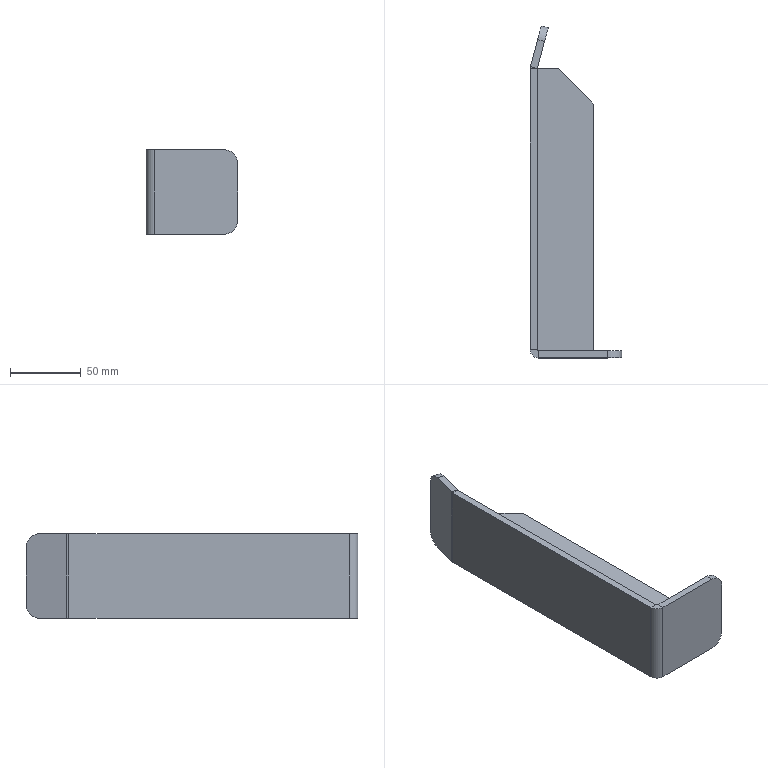Part | SolidWorks | features Fillet 1, FlatPattern 1, Gusset 1, SMBaseFlange 1, SheetMetal 1 | 2 solids | 33 faces | box 65 x 235.272 x 60 mm | volume 126254 mm3 | plane 25 | cylinder 8 | commonest cylinder face diameters 20 x4 2 x2 12 x2
STEP:
#1=CARTESIAN_POINT('',(0.,199.868,60.));
#2=VERTEX_POINT('',#1);
#3=CARTESIAN_POINT('',(-5.,199.868,60.));
#4=VERTEX_POINT('',#3);
#5=CARTESIAN_POINT('',(0.,199.868,60.));
#6=DIRECTION('',(-1.,0.,0.));
#7=VECTOR('',#6,1000.);
#8=LINE('',#5,#7);
#9=EDGE_CURVE('',#2,#4,#8,.T.);
#10=ORIENTED_EDGE('',*,*,#9,.F.);
#11=CARTESIAN_POINT('',(0.03407,200.127,60.));
#12=VERTEX_POINT('',#11);
#13=CARTESIAN_POINT('',(1.,199.868,60.));
#14=DIRECTION('',(0.,0.,1.));
#15=DIRECTION('',(-1.,0.,0.));
#16=AXIS2_PLACEMENT_3D('',#13,#14,#15);
#17=CIRCLE('',#16,1.);
#18=EDGE_CURVE('',#12,#2,#17,.T.);
#19=ORIENTED_EDGE('',*,*,#18,.F.);
#20=CARTESIAN_POINT('',(-4.796,201.421,60.));
#21=VERTEX_POINT('',#20);
#22=CARTESIAN_POINT('',(-4.796,201.421,60.));
#23=DIRECTION('',(0.9659,-0.2588,0.));
#24=VECTOR('',#23,1000.);
#25=LINE('',#22,#24);
#26=EDGE_CURVE('',#21,#12,#25,.T.);
#27=ORIENTED_EDGE('',*,*,#26,.F.);
#28=CARTESIAN_POINT('',(1.,199.868,60.));
#29=DIRECTION('',(0.,0.,1.));
#30=DIRECTION('',(1.,0.,0.));
#31=AXIS2_PLACEMENT_3D('',#28,#29,#30);
#32=CIRCLE('',#31,6.);
#33=EDGE_CURVE('',#21,#4,#32,.T.);
#34=ORIENTED_EDGE('',*,*,#33,.T.);
#35=EDGE_LOOP('',(#10,#19,#27,#34));
#36=FACE_OUTER_BOUND('',#35,.T.);
#37=CARTESIAN_POINT('',(0.,199.868,60.));
#38=DIRECTION('',(0.,0.,1.));
#39=DIRECTION('',(1.,0.,0.));
#40=AXIS2_PLACEMENT_3D('',#37,#38,#39);
#41=PLANE('',#40);
#42=ADVANCED_FACE('',(#36),#41,.T.);
#43=CARTESIAN_POINT('',(0.,1.,60.));
#44=VERTEX_POINT('',#43);
#45=CARTESIAN_POINT('',(0.,200.,60.));
#46=DIRECTION('',(0.,-1.,0.));
#47=VECTOR('',#46,1000.);
#48=LINE('',#45,#47);
#49=EDGE_CURVE('',#2,#44,#48,.T.);
#50=ORIENTED_EDGE('',*,*,#49,.F.);
#51=ORIENTED_EDGE('',*,*,#9,.T.);
#52=CARTESIAN_POINT('',(-5.,1.,60.));
#53=VERTEX_POINT('',#52);
#54=CARTESIAN_POINT('',(-5.,200.,60.));
#55=DIRECTION('',(0.,-1.,0.));
#56=VECTOR('',#55,1000.);
#57=LINE('',#54,#56);
#58=EDGE_CURVE('',#4,#53,#57,.T.);
#59=ORIENTED_EDGE('',*,*,#58,.T.);
#60=CARTESIAN_POINT('',(-5.,1.,60.));
#61=DIRECTION('',(1.,0.,0.));
#62=VECTOR('',#61,1000.);
#63=LINE('',#60,#62);
#64=EDGE_CURVE('',#53,#44,#63,.T.);
#65=ORIENTED_EDGE('',*,*,#64,.T.);
#66=EDGE_LOOP('',(#50,#51,#59,#65));
#67=FACE_OUTER_BOUND('',#66,.T.);
#68=CARTESIAN_POINT('',(-4.796,201.421,60.));
#69=DIRECTION('',(0.,0.,1.));
#70=DIRECTION('',(1.,0.,0.));
#71=AXIS2_PLACEMENT_3D('',#68,#69,#70);
#72=PLANE('',#71);
#73=ADVANCED_FACE('',(#67),#72,.T.);
#74=CARTESIAN_POINT('',(0.03407,200.127,0.));
#75=VERTEX_POINT('',#74);
#76=CARTESIAN_POINT('',(-4.796,201.421,0.));
#77=VERTEX_POINT('',#76);
#78=CARTESIAN_POINT('',(0.03407,200.127,0.));
#79=DIRECTION('',(-0.9659,0.2588,0.));
#80=VECTOR('',#79,1000.);
#81=LINE('',#78,#80);
#82=EDGE_CURVE('',#75,#77,#81,.T.);
#83=ORIENTED_EDGE('',*,*,#82,.F.);
#84=CARTESIAN_POINT('',(0.,199.868,0.));
#85=VERTEX_POINT('',#84);
#86=CARTESIAN_POINT('',(1.,199.868,0.));
#87=DIRECTION('',(0.,0.,1.));
#88=DIRECTION('',(-1.,0.,0.));
#89=AXIS2_PLACEMENT_3D('',#86,#87,#88);
#90=CIRCLE('',#89,1.);
#91=EDGE_CURVE('',#75,#85,#90,.T.);
#92=ORIENTED_EDGE('',*,*,#91,.T.);
#93=CARTESIAN_POINT('',(-5.,199.868,0.));
#94=VERTEX_POINT('',#93);
#95=CARTESIAN_POINT('',(-5.,199.868,0.));
#96=DIRECTION('',(1.,0.,0.));
#97=VECTOR('',#96,1000.);
#98=LINE('',#95,#97);
#99=EDGE_CURVE('',#94,#85,#98,.T.);
#100=ORIENTED_EDGE('',*,*,#99,.F.);
#101=CARTESIAN_POINT('',(1.,199.868,0.));
#102=DIRECTION('',(0.,0.,1.));
#103=DIRECTION('',(1.,0.,0.));
#104=AXIS2_PLACEMENT_3D('',#101,#102,#103);
#105=CIRCLE('',#104,6.);
#106=EDGE_CURVE('',#77,#94,#105,.T.);
#107=ORIENTED_EDGE('',*,*,#106,.F.);
#108=EDGE_LOOP('',(#83,#92,#100,#107));
#109=FACE_OUTER_BOUND('',#108,.T.);
#110=CARTESIAN_POINT('',(0.03407,200.127,0.));
#111=DIRECTION('',(0.,0.,-1.));
#112=DIRECTION('',(-1.,0.,0.));
#113=AXIS2_PLACEMENT_3D('',#110,#111,#112);
#114=PLANE('',#113);
#115=ADVANCED_FACE('',(#109),#114,.T.);
#116=CARTESIAN_POINT('',(0.3468,220.613,0.));
#117=VERTEX_POINT('',#116);
#118=CARTESIAN_POINT('',(-4.83,201.294,0.));
#119=DIRECTION('',(-0.2588,-0.9659,0.));
#120=VECTOR('',#119,1000.);
#121=LINE('',#118,#120);
#122=EDGE_CURVE('',#117,#77,#121,.T.);
#123=ORIENTED_EDGE('',*,*,#122,.F.);
#124=CARTESIAN_POINT('',(5.176,219.319,0.));
#125=VERTEX_POINT('',#124);
#126=CARTESIAN_POINT('',(0.5442,220.56,0.));
#127=DIRECTION('',(0.9659,-0.2588,0.));
#128=VECTOR('',#127,1000.);
#129=LINE('',#126,#128);
#130=EDGE_CURVE('',#117,#125,#129,.T.);
#131=ORIENTED_EDGE('',*,*,#130,.T.);
#132=CARTESIAN_POINT('',(0.,200.,0.));
#133=DIRECTION('',(-0.2588,-0.9659,0.));
#134=VECTOR('',#133,1000.);
#135=LINE('',#132,#134);
#136=EDGE_CURVE('',#125,#75,#135,.T.);
#137=ORIENTED_EDGE('',*,*,#136,.T.);
#138=ORIENTED_EDGE('',*,*,#82,.T.);
#139=EDGE_LOOP('',(#123,#131,#137,#138));
#140=FACE_OUTER_BOUND('',#139,.T.);
#141=CARTESIAN_POINT('',(-5.,199.868,0.));
#142=DIRECTION('',(0.,0.,-1.));
#143=DIRECTION('',(-1.,0.,0.));
#144=AXIS2_PLACEMENT_3D('',#141,#142,#143);
#145=PLANE('',#144);
#146=ADVANCED_FACE('',(#140),#145,.T.);
#147=CARTESIAN_POINT('',(1.,0.,60.));
#148=VERTEX_POINT('',#147);
#149=CARTESIAN_POINT('',(1.,-5.,60.));
#150=VERTEX_POINT('',#149);
#151=CARTESIAN_POINT('',(1.,0.,60.));
#152=DIRECTION('',(0.,-1.,0.));
#153=VECTOR('',#152,1000.);
#154=LINE('',#151,#153);
#155=EDGE_CURVE('',#148,#150,#154,.T.);
#156=ORIENTED_EDGE('',*,*,#155,.F.);
#157=CARTESIAN_POINT('',(1.,1.,60.));
#158=DIRECTION('',(0.,0.,1.));
#159=DIRECTION('',(-1.,0.,0.));
#160=AXIS2_PLACEMENT_3D('',#157,#158,#159);
#161=CIRCLE('',#160,1.);
#162=EDGE_CURVE('',#44,#148,#161,.T.);
#163=ORIENTED_EDGE('',*,*,#162,.F.);
#164=ORIENTED_EDGE('',*,*,#64,.F.);
#165=CARTESIAN_POINT('',(1.,1.,60.));
#166=DIRECTION('',(0.,0.,1.));
#167=DIRECTION('',(1.,0.,0.));
#168=AXIS2_PLACEMENT_3D('',#165,#166,#167);
#169=CIRCLE('',#168,6.);
#170=EDGE_CURVE('',#53,#150,#169,.T.);
#171=ORIENTED_EDGE('',*,*,#170,.T.);
#172=EDGE_LOOP('',(#156,#163,#164,#171));
#173=FACE_OUTER_BOUND('',#172,.T.);
#174=CARTESIAN_POINT('',(1.,0.,60.));
#175=DIRECTION('',(0.,0.,1.));
#176=DIRECTION('',(1.,0.,0.));
#177=AXIS2_PLACEMENT_3D('',#174,#175,#176);
#178=PLANE('',#177);
#179=ADVANCED_FACE('',(#173),#178,.T.);
#180=CARTESIAN_POINT('',(50.,-5.,60.));
#181=VERTEX_POINT('',#180);
#182=CARTESIAN_POINT('',(0.,-5.,60.));
#183=DIRECTION('',(1.,0.,0.));
#184=VECTOR('',#183,1000.);
#185=LINE('',#182,#184);
#186=EDGE_CURVE('',#150,#181,#185,.T.);
#187=ORIENTED_EDGE('',*,*,#186,.T.);
#188=CARTESIAN_POINT('',(50.,0.,60.));
#189=VERTEX_POINT('',#188);
#190=CARTESIAN_POINT('',(50.,1.,60.));
#191=DIRECTION('',(0.,1.,0.));
#192=VECTOR('',#191,1000.);
#193=LINE('',#190,#192);
#194=EDGE_CURVE('',#181,#189,#193,.T.);
#195=ORIENTED_EDGE('',*,*,#194,.T.);
#196=CARTESIAN_POINT('',(0.,0.,60.));
#197=DIRECTION('',(1.,0.,0.));
#198=VECTOR('',#197,1000.);
#199=LINE('',#196,#198);
#200=EDGE_CURVE('',#148,#189,#199,.T.);
#201=ORIENTED_EDGE('',*,*,#200,.F.);
#202=ORIENTED_EDGE('',*,*,#155,.T.);
#203=EDGE_LOOP('',(#187,#195,#201,#202));
#204=FACE_OUTER_BOUND('',#203,.T.);
#205=CARTESIAN_POINT('',(-5.,1.,60.));
#206=DIRECTION('',(0.,0.,1.));
#207=DIRECTION('',(1.,0.,0.));
#208=AXIS2_PLACEMENT_3D('',#205,#206,#207);
#209=PLANE('',#208);
#210=ADVANCED_FACE('',(#204),#209,.T.);
#211=CARTESIAN_POINT('',(0.,1.,0.));
#212=VERTEX_POINT('',#211);
#213=CARTESIAN_POINT('',(-5.,1.,0.));
#214=VERTEX_POINT('',#213);
#215=CARTESIAN_POINT('',(0.,1.,0.));
#216=DIRECTION('',(-1.,0.,0.));
#217=VECTOR('',#216,1000.);
#218=LINE('',#215,#217);
#219=EDGE_CURVE('',#212,#214,#218,.T.);
#220=ORIENTED_EDGE('',*,*,#219,.F.);
#221=CARTESIAN_POINT('',(1.,0.,0.));
#222=VERTEX_POINT('',#221);
#223=CARTESIAN_POINT('',(1.,1.,0.));
#224=DIRECTION('',(0.,0.,1.));
#225=DIRECTION('',(-1.,0.,0.));
#226=AXIS2_PLACEMENT_3D('',#223,#224,#225);
#227=CIRCLE('',#226,1.);
#228=EDGE_CURVE('',#212,#222,#227,.T.);
#229=ORIENTED_EDGE('',*,*,#228,.T.);
#230=CARTESIAN_POINT('',(1.,-5.,0.));
#231=VERTEX_POINT('',#230);
#232=CARTESIAN_POINT('',(1.,-5.,0.));
#233=DIRECTION('',(0.,1.,0.));
#234=VECTOR('',#233,1000.);
#235=LINE('',#232,#234);
#236=EDGE_CURVE('',#231,#222,#235,.T.);
#237=ORIENTED_EDGE('',*,*,#236,.F.);
#238=CARTESIAN_POINT('',(1.,1.,0.));
#239=DIRECTION('',(0.,0.,1.));
#240=DIRECTION('',(1.,0.,0.));
#241=AXIS2_PLACEMENT_3D('',#238,#239,#240);
#242=CIRCLE('',#241,6.);
#243=EDGE_CURVE('',#214,#231,#242,.T.);
#244=ORIENTED_EDGE('',*,*,#243,.F.);
#245=EDGE_LOOP('',(#220,#229,#237,#244));
#246=FACE_OUTER_BOUND('',#245,.T.);
#247=CARTESIAN_POINT('',(0.,1.,0.));
#248=DIRECTION('',(0.,0.,-1.));
#249=DIRECTION('',(-1.,0.,0.));
#250=AXIS2_PLACEMENT_3D('',#247,#248,#249);
#251=PLANE('',#250);
#252=ADVANCED_FACE('',(#246),#251,.T.);
#253=CARTESIAN_POINT('',(0.,200.,0.));
#254=DIRECTION('',(0.,-1.,0.));
#255=VECTOR('',#254,1000.);
#256=LINE('',#253,#255);
#257=EDGE_CURVE('',#85,#212,#256,.T.);
#258=ORIENTED_EDGE('',*,*,#257,.T.);
#259=ORIENTED_EDGE('',*,*,#219,.T.);
#260=CARTESIAN_POINT('',(-5.,200.,0.));
#261=DIRECTION('',(0.,-1.,0.));
#262=VECTOR('',#261,1000.);
#263=LINE('',#260,#262);
#264=EDGE_CURVE('',#94,#214,#263,.T.);
#265=ORIENTED_EDGE('',*,*,#264,.F.);
#266=ORIENTED_EDGE('',*,*,#99,.T.);
#267=EDGE_LOOP('',(#258,#259,#265,#266));
#268=FACE_OUTER_BOUND('',#267,.T.);
#269=CARTESIAN_POINT('',(1.,-5.,0.));
#270=DIRECTION('',(0.,0.,-1.));
#271=DIRECTION('',(-1.,0.,0.));
#272=AXIS2_PLACEMENT_3D('',#269,#270,#271);
#273=PLANE('',#272);
#274=ADVANCED_FACE('',(#268),#273,.T.);
#275=CARTESIAN_POINT('',(50.,-5.,0.));
#276=VERTEX_POINT('',#275);
#277=CARTESIAN_POINT('',(0.,-5.,0.));
#278=DIRECTION('',(1.,0.,0.));
#279=VECTOR('',#278,1000.);
#280=LINE('',#277,#279);
#281=EDGE_CURVE('',#231,#276,#280,.T.);
#282=ORIENTED_EDGE('',*,*,#281,.T.);
#283=CARTESIAN_POINT('',(60.,-5.,10.));
#284=VERTEX_POINT('',#283);
#285=CARTESIAN_POINT('',(50.,-5.,10.));
#286=DIRECTION('',(0.,-1.,0.));
#287=DIRECTION('',(0.,0.,1.));
#288=AXIS2_PLACEMENT_3D('',#285,#286,#287);
#289=CIRCLE('',#288,10.);
#290=EDGE_CURVE('',#276,#284,#289,.T.);
#291=ORIENTED_EDGE('',*,*,#290,.T.);
#292=CARTESIAN_POINT('',(60.,-5.,50.));
#293=VERTEX_POINT('',#292);
#294=CARTESIAN_POINT('',(60.,-5.,60.));
#295=DIRECTION('',(0.,0.,-1.));
#296=VECTOR('',#295,1000.);
#297=LINE('',#294,#296);
#298=EDGE_CURVE('',#293,#284,#297,.T.);
#299=ORIENTED_EDGE('',*,*,#298,.F.);
#300=CARTESIAN_POINT('',(50.,-5.,50.));
#301=DIRECTION('',(0.,-1.,0.));
#302=DIRECTION('',(0.,0.,1.));
#303=AXIS2_PLACEMENT_3D('',#300,#301,#302);
#304=CIRCLE('',#303,10.);
#305=EDGE_CURVE('',#293,#181,#304,.T.);
#306=ORIENTED_EDGE('',*,*,#305,.T.);
#307=ORIENTED_EDGE('',*,*,#186,.F.);
#308=CARTESIAN_POINT('',(1.,-5.,60.));
#309=DIRECTION('',(0.,0.,-1.));
#310=VECTOR('',#309,1000.);
#311=LINE('',#308,#310);
#312=EDGE_CURVE('',#150,#231,#311,.T.);
#313=ORIENTED_EDGE('',*,*,#312,.T.);
#314=EDGE_LOOP('',(#282,#291,#299,#306,#307,#313));
#315=FACE_OUTER_BOUND('',#314,.T.);
#316=CARTESIAN_POINT('',(0.,-5.,60.));
#317=DIRECTION('',(0.,1.,0.));
#318=DIRECTION('',(0.,0.,1.));
#319=AXIS2_PLACEMENT_3D('',#316,#317,#318);
#320=PLANE('',#319);
#321=ADVANCED_FACE('',(#315),#320,.F.);
#322=ORIENTED_EDGE('',*,*,#298,.T.);
#323=CARTESIAN_POINT('',(60.,0.,10.));
#324=VERTEX_POINT('',#323);
#325=CARTESIAN_POINT('',(60.,0.,10.));
#326=DIRECTION('',(0.,1.,0.));
#327=VECTOR('',#326,1000.);
#328=LINE('',#325,#327);
#329=EDGE_CURVE('',#284,#324,#328,.T.);
#330=ORIENTED_EDGE('',*,*,#329,.T.);
#331=CARTESIAN_POINT('',(60.,0.,50.));
#332=VERTEX_POINT('',#331);
#333=CARTESIAN_POINT('',(60.,0.,60.));
#334=DIRECTION('',(0.,0.,-1.));
#335=VECTOR('',#334,1000.);
#336=LINE('',#333,#335);
#337=EDGE_CURVE('',#332,#324,#336,.T.);
#338=ORIENTED_EDGE('',*,*,#337,.F.);
#339=CARTESIAN_POINT('',(60.,0.,50.));
#340=DIRECTION('',(0.,-1.,0.));
#341=VECTOR('',#340,1000.);
#342=LINE('',#339,#341);
#343=EDGE_CURVE('',#332,#293,#342,.T.);
#344=ORIENTED_EDGE('',*,*,#343,.T.);
#345=EDGE_LOOP('',(#322,#330,#338,#344));
#346=FACE_OUTER_BOUND('',#345,.T.);
#347=CARTESIAN_POINT('',(60.,0.,60.));
#348=DIRECTION('',(1.,0.,0.));
#349=DIRECTION('',(0.,0.,-1.));
#350=AXIS2_PLACEMENT_3D('',#347,#348,#349);
#351=PLANE('',#350);
#352=ADVANCED_FACE('',(#346),#351,.T.);
#353=ORIENTED_EDGE('',*,*,#337,.T.);
#354=CARTESIAN_POINT('',(50.,0.,0.));
#355=VERTEX_POINT('',#354);
#356=CARTESIAN_POINT('',(50.,0.,10.));
#357=DIRECTION('',(0.,1.,0.));
#358=DIRECTION('',(0.,0.,1.));
#359=AXIS2_PLACEMENT_3D('',#356,#357,#358);
#360=CIRCLE('',#359,10.);
#361=EDGE_CURVE('',#324,#355,#360,.T.);
#362=ORIENTED_EDGE('',*,*,#361,.T.);
#363=CARTESIAN_POINT('',(0.,0.,0.));
#364=DIRECTION('',(1.,0.,0.));
#365=VECTOR('',#364,1000.);
#366=LINE('',#363,#365);
#367=EDGE_CURVE('',#222,#355,#366,.T.);
#368=ORIENTED_EDGE('',*,*,#367,.F.);
#369=CARTESIAN_POINT('',(1.,0.,60.));
#370=DIRECTION('',(0.,0.,-1.));
#371=VECTOR('',#370,1000.);
#372=LINE('',#369,#371);
#373=EDGE_CURVE('',#148,#222,#372,.T.);
#374=ORIENTED_EDGE('',*,*,#373,.F.);
#375=ORIENTED_EDGE('',*,*,#200,.T.);
#376=CARTESIAN_POINT('',(50.,0.,50.));
#377=DIRECTION('',(0.,1.,0.));
#378=DIRECTION('',(0.,0.,1.));
#379=AXIS2_PLACEMENT_3D('',#376,#377,#378);
#380=CIRCLE('',#379,10.);
#381=EDGE_CURVE('',#189,#332,#380,.T.);
#382=ORIENTED_EDGE('',*,*,#381,.T.);
#383=EDGE_LOOP('',(#353,#362,#368,#374,#375,#382));
#384=FACE_OUTER_BOUND('',#383,.T.);
#385=CARTESIAN_POINT('',(0.,0.,60.));
#386=DIRECTION('',(0.,1.,0.));
#387=DIRECTION('',(0.,0.,1.));
#388=AXIS2_PLACEMENT_3D('',#385,#386,#387);
#389=PLANE('',#388);
#390=ADVANCED_FACE('',(#384),#389,.T.);
#391=ORIENTED_EDGE('',*,*,#228,.F.);
#392=CARTESIAN_POINT('',(0.,1.,60.));
#393=DIRECTION('',(0.,0.,-1.));
#394=VECTOR('',#393,1000.);
#395=LINE('',#392,#394);
#396=EDGE_CURVE('',#44,#212,#395,.T.);
#397=ORIENTED_EDGE('',*,*,#396,.F.);
#398=ORIENTED_EDGE('',*,*,#162,.T.);
#399=ORIENTED_EDGE('',*,*,#373,.T.);
#400=EDGE_LOOP('',(#391,#397,#398,#399));
#401=FACE_OUTER_BOUND('',#400,.T.);
#402=CARTESIAN_POINT('',(1.,1.,60.));
#403=DIRECTION('',(0.,0.,-1.));
#404=DIRECTION('',(-1.,0.,0.));
#405=AXIS2_PLACEMENT_3D('',#402,#403,#404);
#406=CYLINDRICAL_SURFACE('',#405,1.);
#407=ADVANCED_FACE('',(#401),#406,.F.);
#408=ORIENTED_EDGE('',*,*,#257,.F.);
#409=CARTESIAN_POINT('',(0.,199.868,60.));
#410=DIRECTION('',(0.,0.,-1.));
#411=VECTOR('',#410,1000.);
#412=LINE('',#409,#411);
#413=EDGE_CURVE('',#2,#85,#412,.T.);
#414=ORIENTED_EDGE('',*,*,#413,.F.);
#415=ORIENTED_EDGE('',*,*,#49,.T.);
#416=ORIENTED_EDGE('',*,*,#396,.T.);
#417=EDGE_LOOP('',(#408,#414,#415,#416));
#418=FACE_OUTER_BOUND('',#417,.T.);
#419=CARTESIAN_POINT('',(0.,200.,60.));
#420=DIRECTION('',(1.,0.,0.));
#421=DIRECTION('',(0.,1.,0.));
#422=AXIS2_PLACEMENT_3D('',#419,#420,#421);
#423=PLANE('',#422);
#424=ADVANCED_FACE('',(#418),#423,.T.);
#425=ORIENTED_EDGE('',*,*,#91,.F.);
#426=CARTESIAN_POINT('',(0.03407,200.127,60.));
#427=DIRECTION('',(0.,0.,-1.));
#428=VECTOR('',#427,1000.);
#429=LINE('',#426,#428);
#430=EDGE_CURVE('',#12,#75,#429,.T.);
#431=ORIENTED_EDGE('',*,*,#430,.F.);
#432=ORIENTED_EDGE('',*,*,#18,.T.);
#433=ORIENTED_EDGE('',*,*,#413,.T.);
#434=EDGE_LOOP('',(#425,#431,#432,#433));
#435=FACE_OUTER_BOUND('',#434,.T.);
#436=CARTESIAN_POINT('',(1.,199.868,60.));
#437=DIRECTION('',(0.,0.,-1.));
#438=DIRECTION('',(-1.,0.,0.));
#439=AXIS2_PLACEMENT_3D('',#436,#437,#438);
#440=CYLINDRICAL_SURFACE('',#439,1.);
#441=ADVANCED_FACE('',(#435),#440,.F.);
#442=ORIENTED_EDGE('',*,*,#136,.F.);
#443=CARTESIAN_POINT('',(7.765,228.978,10.));
#444=VERTEX_POINT('',#443);
#445=CARTESIAN_POINT('',(5.176,219.319,10.));
#446=DIRECTION('',(0.9659,-0.2588,0.));
#447=DIRECTION('',(0.2588,0.9659,0.));
#448=AXIS2_PLACEMENT_3D('',#445,#446,#447);
#449=CIRCLE('',#448,10.);
#450=EDGE_CURVE('',#125,#444,#449,.T.);
#451=ORIENTED_EDGE('',*,*,#450,.T.);
#452=CARTESIAN_POINT('',(7.765,228.978,50.));
#453=VERTEX_POINT('',#452);
#454=CARTESIAN_POINT('',(7.765,228.978,60.));
#455=DIRECTION('',(0.,0.,-1.));
#456=VECTOR('',#455,1000.);
#457=LINE('',#454,#456);
#458=EDGE_CURVE('',#453,#444,#457,.T.);
#459=ORIENTED_EDGE('',*,*,#458,.F.);
#460=CARTESIAN_POINT('',(5.176,219.319,60.));
#461=VERTEX_POINT('',#460);
#462=CARTESIAN_POINT('',(5.176,219.319,50.));
#463=DIRECTION('',(0.9659,-0.2588,0.));
#464=DIRECTION('',(0.2588,0.9659,0.));
#465=AXIS2_PLACEMENT_3D('',#462,#463,#464);
#466=CIRCLE('',#465,10.);
#467=EDGE_CURVE('',#453,#461,#466,.T.);
#468=ORIENTED_EDGE('',*,*,#467,.T.);
#469=CARTESIAN_POINT('',(0.,200.,60.));
#470=DIRECTION('',(-0.2588,-0.9659,0.));
#471=VECTOR('',#470,1000.);
#472=LINE('',#469,#471);
#473=EDGE_CURVE('',#461,#12,#472,.T.);
#474=ORIENTED_EDGE('',*,*,#473,.T.);
#475=ORIENTED_EDGE('',*,*,#430,.T.);
#476=EDGE_LOOP('',(#442,#451,#459,#468,#474,#475));
#477=FACE_OUTER_BOUND('',#476,.T.);
#478=CARTESIAN_POINT('',(0.,200.,60.));
#479=DIRECTION('',(0.9659,-0.2588,0.));
#480=DIRECTION('',(0.2588,0.9659,0.));
#481=AXIS2_PLACEMENT_3D('',#478,#479,#480);
#482=PLANE('',#481);
#483=ADVANCED_FACE('',(#477),#482,.T.);
#484=ORIENTED_EDGE('',*,*,#458,.T.);
#485=CARTESIAN_POINT('',(2.935,230.272,10.));
#486=VERTEX_POINT('',#485);
#487=CARTESIAN_POINT('',(2.935,230.272,10.));
#488=DIRECTION('',(-0.9659,0.2588,0.));
#489=VECTOR('',#488,1000.);
#490=LINE('',#487,#489);
#491=EDGE_CURVE('',#444,#486,#490,.T.);
#492=ORIENTED_EDGE('',*,*,#491,.T.);
#493=CARTESIAN_POINT('',(2.935,230.272,50.));
#494=VERTEX_POINT('',#493);
#495=CARTESIAN_POINT('',(2.935,230.272,60.));
#496=DIRECTION('',(0.,0.,-1.));
#497=VECTOR('',#496,1000.);
#498=LINE('',#495,#497);
#499=EDGE_CURVE('',#494,#486,#498,.T.);
#500=ORIENTED_EDGE('',*,*,#499,.F.);
#501=CARTESIAN_POINT('',(7.765,228.978,50.));
#502=DIRECTION('',(0.9659,-0.2588,0.));
#503=VECTOR('',#502,1000.);
#504=LINE('',#501,#503);
#505=EDGE_CURVE('',#494,#453,#504,.T.);
#506=ORIENTED_EDGE('',*,*,#505,.T.);
#507=EDGE_LOOP('',(#484,#492,#500,#506));
#508=FACE_OUTER_BOUND('',#507,.T.);
#509=CARTESIAN_POINT('',(2.935,230.272,60.));
#510=DIRECTION('',(0.2588,0.9659,0.));
#511=DIRECTION('',(-0.9659,0.2588,0.));
#512=AXIS2_PLACEMENT_3D('',#509,#510,#511);
#513=PLANE('',#512);
#514=ADVANCED_FACE('',(#508),#513,.T.);
#515=ORIENTED_EDGE('',*,*,#499,.T.);
#516=CARTESIAN_POINT('',(0.3468,220.613,10.));
#517=DIRECTION('',(-0.9659,0.2588,0.));
#518=DIRECTION('',(0.2588,0.9659,0.));
#519=AXIS2_PLACEMENT_3D('',#516,#517,#518);
#520=CIRCLE('',#519,10.);
#521=EDGE_CURVE('',#486,#117,#520,.T.);
#522=ORIENTED_EDGE('',*,*,#521,.T.);
#523=ORIENTED_EDGE('',*,*,#122,.T.);
#524=CARTESIAN_POINT('',(-4.796,201.421,60.));
#525=DIRECTION('',(0.,0.,-1.));
#526=VECTOR('',#525,1000.);
#527=LINE('',#524,#526);
#528=EDGE_CURVE('',#21,#77,#527,.T.);
#529=ORIENTED_EDGE('',*,*,#528,.F.);
#530=CARTESIAN_POINT('',(0.3468,220.613,60.));
#531=VERTEX_POINT('',#530);
#532=CARTESIAN_POINT('',(-4.83,201.294,60.));
#533=DIRECTION('',(-0.2588,-0.9659,0.));
#534=VECTOR('',#533,1000.);
#535=LINE('',#532,#534);
#536=EDGE_CURVE('',#531,#21,#535,.T.);
#537=ORIENTED_EDGE('',*,*,#536,.F.);
#538=CARTESIAN_POINT('',(0.3468,220.613,50.));
#539=DIRECTION('',(-0.9659,0.2588,0.));
#540=DIRECTION('',(0.2588,0.9659,0.));
#541=AXIS2_PLACEMENT_3D('',#538,#539,#540);
#542=CIRCLE('',#541,10.);
#543=EDGE_CURVE('',#531,#494,#542,.T.);
#544=ORIENTED_EDGE('',*,*,#543,.T.);
#545=EDGE_LOOP('',(#515,#522,#523,#529,#537,#544));
#546=FACE_OUTER_BOUND('',#545,.T.);
#547=CARTESIAN_POINT('',(-4.83,201.294,60.));
#548=DIRECTION('',(0.9659,-0.2588,0.));
#549=DIRECTION('',(0.2588,0.9659,0.));
#550=AXIS2_PLACEMENT_3D('',#547,#548,#549);
#551=PLANE('',#550);
#552=ADVANCED_FACE('',(#546),#551,.F.);
#553=ORIENTED_EDGE('',*,*,#106,.T.);
#554=CARTESIAN_POINT('',(-5.,199.868,60.));
#555=DIRECTION('',(0.,0.,-1.));
#556=VECTOR('',#555,1000.);
#557=LINE('',#554,#556);
#558=EDGE_CURVE('',#4,#94,#557,.T.);
#559=ORIENTED_EDGE('',*,*,#558,.F.);
#560=ORIENTED_EDGE('',*,*,#33,.F.);
#561=ORIENTED_EDGE('',*,*,#528,.T.);
#562=EDGE_LOOP('',(#553,#559,#560,#561));
#563=FACE_OUTER_BOUND('',#562,.T.);
#564=CARTESIAN_POINT('',(1.,199.868,60.));
#565=DIRECTION('',(0.,0.,-1.));
#566=DIRECTION('',(-1.,0.,0.));
#567=AXIS2_PLACEMENT_3D('',#564,#565,#566);
#568=CYLINDRICAL_SURFACE('',#567,6.);
#569=ADVANCED_FACE('',(#563),#568,.T.);
#570=ORIENTED_EDGE('',*,*,#264,.T.);
#571=CARTESIAN_POINT('',(-5.,1.,60.));
#572=DIRECTION('',(0.,0.,-1.));
#573=VECTOR('',#572,1000.);
#574=LINE('',#571,#573);
#575=EDGE_CURVE('',#53,#214,#574,.T.);
#576=ORIENTED_EDGE('',*,*,#575,.F.);
#577=ORIENTED_EDGE('',*,*,#58,.F.);
#578=ORIENTED_EDGE('',*,*,#558,.T.);
#579=EDGE_LOOP('',(#570,#576,#577,#578));
#580=FACE_OUTER_BOUND('',#579,.T.);
#581=CARTESIAN_POINT('',(-5.,200.,60.));
#582=DIRECTION('',(1.,0.,0.));
#583=DIRECTION('',(0.,1.,0.));
#584=AXIS2_PLACEMENT_3D('',#581,#582,#583);
#585=PLANE('',#584);
#586=ADVANCED_FACE('',(#580),#585,.F.);
#587=ORIENTED_EDGE('',*,*,#243,.T.);
#588=ORIENTED_EDGE('',*,*,#312,.F.);
#589=ORIENTED_EDGE('',*,*,#170,.F.);
#590=ORIENTED_EDGE('',*,*,#575,.T.);
#591=EDGE_LOOP('',(#587,#588,#589,#590));
#592=FACE_OUTER_BOUND('',#591,.T.);
#593=CARTESIAN_POINT('',(1.,1.,60.));
#594=DIRECTION('',(0.,0.,-1.));
#595=DIRECTION('',(-1.,0.,0.));
#596=AXIS2_PLACEMENT_3D('',#593,#594,#595);
#597=CYLINDRICAL_SURFACE('',#596,6.);
#598=ADVANCED_FACE('',(#592),#597,.T.);
#599=ORIENTED_EDGE('',*,*,#473,.F.);
#600=CARTESIAN_POINT('',(0.3468,220.613,60.));
#601=DIRECTION('',(-0.9659,0.2588,0.));
#602=VECTOR('',#601,1000.);
#603=LINE('',#600,#602);
#604=EDGE_CURVE('',#461,#531,#603,.T.);
#605=ORIENTED_EDGE('',*,*,#604,.T.);
#606=ORIENTED_EDGE('',*,*,#536,.T.);
#607=ORIENTED_EDGE('',*,*,#26,.T.);
#608=EDGE_LOOP('',(#599,#605,#606,#607));
#609=FACE_OUTER_BOUND('',#608,.T.);
#610=CARTESIAN_POINT('',(1.,1.,60.));
#611=DIRECTION('',(0.,0.,-1.));
#612=DIRECTION('',(-1.,0.,0.));
#613=AXIS2_PLACEMENT_3D('',#610,#611,#612);
#614=PLANE('',#613);
#615=ADVANCED_FACE('',(#609),#614,.F.);
#616=ORIENTED_EDGE('',*,*,#367,.T.);
#617=CARTESIAN_POINT('',(50.,1.,0.));
#618=DIRECTION('',(0.,-1.,0.));
#619=VECTOR('',#618,1000.);
#620=LINE('',#617,#619);
#621=EDGE_CURVE('',#355,#276,#620,.T.);
#622=ORIENTED_EDGE('',*,*,#621,.T.);
#623=ORIENTED_EDGE('',*,*,#281,.F.);
#624=ORIENTED_EDGE('',*,*,#236,.T.);
#625=EDGE_LOOP('',(#616,#622,#623,#624));
#626=FACE_OUTER_BOUND('',#625,.T.);
#627=CARTESIAN_POINT('',(1.,1.,0.));
#628=DIRECTION('',(0.,0.,-1.));
#629=DIRECTION('',(-1.,0.,0.));
#630=AXIS2_PLACEMENT_3D('',#627,#628,#629);
#631=PLANE('',#630);
#632=ADVANCED_FACE('',(#626),#631,.T.);
#633=ORIENTED_EDGE('',*,*,#361,.F.);
#634=ORIENTED_EDGE('',*,*,#329,.F.);
#635=ORIENTED_EDGE('',*,*,#290,.F.);
#636=ORIENTED_EDGE('',*,*,#621,.F.);
#637=EDGE_LOOP('',(#633,#634,#635,#636));
#638=FACE_OUTER_BOUND('',#637,.T.);
#639=CARTESIAN_POINT('',(50.,1.,10.));
#640=DIRECTION('',(0.,-1.,0.));
#641=DIRECTION('',(0.,0.,-1.));
#642=AXIS2_PLACEMENT_3D('',#639,#640,#641);
#643=CYLINDRICAL_SURFACE('',#642,10.);
#644=ADVANCED_FACE('',(#638),#643,.T.);
#645=ORIENTED_EDGE('',*,*,#381,.F.);
#646=ORIENTED_EDGE('',*,*,#194,.F.);
#647=ORIENTED_EDGE('',*,*,#305,.F.);
#648=ORIENTED_EDGE('',*,*,#343,.F.);
#649=EDGE_LOOP('',(#645,#646,#647,#648));
#650=FACE_OUTER_BOUND('',#649,.T.);
#651=CARTESIAN_POINT('',(50.,0.,50.));
#652=DIRECTION('',(0.,-1.,0.));
#653=DIRECTION('',(0.,0.,-1.));
#654=AXIS2_PLACEMENT_3D('',#651,#652,#653);
#655=CYLINDRICAL_SURFACE('',#654,10.);
#656=ADVANCED_FACE('',(#650),#655,.T.);
#657=ORIENTED_EDGE('',*,*,#521,.F.);
#658=ORIENTED_EDGE('',*,*,#491,.F.);
#659=ORIENTED_EDGE('',*,*,#450,.F.);
#660=ORIENTED_EDGE('',*,*,#130,.F.);
#661=EDGE_LOOP('',(#657,#658,#659,#660));
#662=FACE_OUTER_BOUND('',#661,.T.);
#663=CARTESIAN_POINT('',(0.5442,220.56,10.));
#664=DIRECTION('',(0.9659,-0.2588,0.));
#665=DIRECTION('',(0.2588,0.9659,0.));
#666=AXIS2_PLACEMENT_3D('',#663,#664,#665);
#667=CYLINDRICAL_SURFACE('',#666,10.);
#668=ADVANCED_FACE('',(#662),#667,.T.);
#669=ORIENTED_EDGE('',*,*,#543,.F.);
#670=ORIENTED_EDGE('',*,*,#604,.F.);
#671=ORIENTED_EDGE('',*,*,#467,.F.);
#672=ORIENTED_EDGE('',*,*,#505,.F.);
#673=EDGE_LOOP('',(#669,#670,#671,#672));
#674=FACE_OUTER_BOUND('',#673,.T.);
#675=CARTESIAN_POINT('',(0.3468,220.613,50.));
#676=DIRECTION('',(-0.9659,0.2588,0.));
#677=DIRECTION('',(-0.2588,-0.9659,0.));
#678=AXIS2_PLACEMENT_3D('',#675,#676,#677);
#679=CYLINDRICAL_SURFACE('',#678,10.);
#680=ADVANCED_FACE('',(#674),#679,.T.);
#681=CLOSED_SHELL('',(#42,#73,#115,#146,#179,#210,#252,#274,#321,#352,#390,#407,#424,#441,#483,#514,#552,#569,#586,#598,#615,#632,#644,#656,#668,#680));
#682=MANIFOLD_SOLID_BREP('',#681);
#683=CARTESIAN_POINT('',(0.,200.,32.5));
#684=VERTEX_POINT('',#683);
#685=CARTESIAN_POINT('',(15.,200.,32.5));
#686=VERTEX_POINT('',#685);
#687=CARTESIAN_POINT('',(0.,200.,32.5));
#688=DIRECTION('',(1.,0.,0.));
#689=VECTOR('',#688,1000.);
#690=LINE('',#687,#689);
#691=EDGE_CURVE('',#684,#686,#690,.T.);
#692=ORIENTED_EDGE('',*,*,#691,.T.);
#693=CARTESIAN_POINT('',(15.,200.,27.5));
#694=VERTEX_POINT('',#693);
#695=CARTESIAN_POINT('',(15.,200.,27.5));
#696=DIRECTION('',(0.,0.,1.));
#697=VECTOR('',#696,1000.);
#698=LINE('',#695,#697);
#699=EDGE_CURVE('',#694,#686,#698,.T.);
#700=ORIENTED_EDGE('',*,*,#699,.F.);
#701=CARTESIAN_POINT('',(0.,200.,27.5));
#702=VERTEX_POINT('',#701);
#703=CARTESIAN_POINT('',(0.,200.,27.5));
#704=DIRECTION('',(1.,0.,0.));
#705=VECTOR('',#704,1000.);
#706=LINE('',#703,#705);
#707=EDGE_CURVE('',#702,#694,#706,.T.);
#708=ORIENTED_EDGE('',*,*,#707,.F.);
#709=CARTESIAN_POINT('',(0.,200.,27.5));
#710=DIRECTION('',(0.,0.,1.));
#711=VECTOR('',#710,1000.);
#712=LINE('',#709,#711);
#713=EDGE_CURVE('',#702,#684,#712,.T.);
#714=ORIENTED_EDGE('',*,*,#713,.T.);
#715=EDGE_LOOP('',(#692,#700,#708,#714));
#716=FACE_OUTER_BOUND('',#715,.T.);
#717=CARTESIAN_POINT('',(0.,200.,27.5));
#718=DIRECTION('',(0.,-1.,0.));
#719=DIRECTION('',(0.,0.,-1.));
#720=AXIS2_PLACEMENT_3D('',#717,#718,#719);
#721=PLANE('',#720);
#722=ADVANCED_FACE('',(#716),#721,.F.);
#723=CARTESIAN_POINT('',(40.,175.,32.5));
#724=VERTEX_POINT('',#723);
#725=CARTESIAN_POINT('',(15.,200.,32.5));
#726=DIRECTION('',(0.7071,-0.7071,0.));
#727=VECTOR('',#726,1000.);
#728=LINE('',#725,#727);
#729=EDGE_CURVE('',#686,#724,#728,.T.);
#730=ORIENTED_EDGE('',*,*,#729,.T.);
#731=CARTESIAN_POINT('',(40.,175.,27.5));
#732=VERTEX_POINT('',#731);
#733=CARTESIAN_POINT('',(40.,175.,27.5));
#734=DIRECTION('',(0.,0.,1.));
#735=VECTOR('',#734,1000.);
#736=LINE('',#733,#735);
#737=EDGE_CURVE('',#732,#724,#736,.T.);
#738=ORIENTED_EDGE('',*,*,#737,.F.);
#739=CARTESIAN_POINT('',(15.,200.,27.5));
#740=DIRECTION('',(0.7071,-0.7071,0.));
#741=VECTOR('',#740,1000.);
#742=LINE('',#739,#741);
#743=EDGE_CURVE('',#694,#732,#742,.T.);
#744=ORIENTED_EDGE('',*,*,#743,.F.);
#745=ORIENTED_EDGE('',*,*,#699,.T.);
#746=EDGE_LOOP('',(#730,#738,#744,#745));
#747=FACE_OUTER_BOUND('',#746,.T.);
#748=CARTESIAN_POINT('',(15.,200.,27.5));
#749=DIRECTION('',(-0.7071,-0.7071,0.));
#750=DIRECTION('',(0.7071,-0.7071,0.));
#751=AXIS2_PLACEMENT_3D('',#748,#749,#750);
#752=PLANE('',#751);
#753=ADVANCED_FACE('',(#747),#752,.F.);
#754=CARTESIAN_POINT('',(40.,0.,32.5));
#755=VERTEX_POINT('',#754);
#756=CARTESIAN_POINT('',(40.,0.,32.5));
#757=DIRECTION('',(0.,-1.,0.));
#758=VECTOR('',#757,1000.);
#759=LINE('',#756,#758);
#760=EDGE_CURVE('',#724,#755,#759,.T.);
#761=ORIENTED_EDGE('',*,*,#760,.T.);
#762=CARTESIAN_POINT('',(40.,0.,27.5));
#763=VERTEX_POINT('',#762);
#764=CARTESIAN_POINT('',(40.,0.,27.5));
#765=DIRECTION('',(0.,0.,1.));
#766=VECTOR('',#765,1000.);
#767=LINE('',#764,#766);
#768=EDGE_CURVE('',#763,#755,#767,.T.);
#769=ORIENTED_EDGE('',*,*,#768,.F.);
#770=CARTESIAN_POINT('',(40.,0.,27.5));
#771=DIRECTION('',(0.,-1.,0.));
#772=VECTOR('',#771,1000.);
#773=LINE('',#770,#772);
#774=EDGE_CURVE('',#732,#763,#773,.T.);
#775=ORIENTED_EDGE('',*,*,#774,.F.);
#776=ORIENTED_EDGE('',*,*,#737,.T.);
#777=EDGE_LOOP('',(#761,#769,#775,#776));
#778=FACE_OUTER_BOUND('',#777,.T.);
#779=CARTESIAN_POINT('',(40.,0.,27.5));
#780=DIRECTION('',(-1.,0.,0.));
#781=DIRECTION('',(0.,0.,1.));
#782=AXIS2_PLACEMENT_3D('',#779,#780,#781);
#783=PLANE('',#782);
#784=ADVANCED_FACE('',(#778),#783,.F.);
#785=CARTESIAN_POINT('',(0.,0.,32.5));
#786=VERTEX_POINT('',#785);
#787=CARTESIAN_POINT('',(0.,0.,32.5));
#788=DIRECTION('',(-1.,0.,0.));
#789=VECTOR('',#788,1000.);
#790=LINE('',#787,#789);
#791=EDGE_CURVE('',#755,#786,#790,.T.);
#792=ORIENTED_EDGE('',*,*,#791,.T.);
#793=CARTESIAN_POINT('',(0.,0.,27.5));
#794=VERTEX_POINT('',#793);
#795=CARTESIAN_POINT('',(0.,0.,27.5));
#796=DIRECTION('',(0.,0.,1.));
#797=VECTOR('',#796,1000.);
#798=LINE('',#795,#797);
#799=EDGE_CURVE('',#794,#786,#798,.T.);
#800=ORIENTED_EDGE('',*,*,#799,.F.);
#801=CARTESIAN_POINT('',(0.,0.,27.5));
#802=DIRECTION('',(-1.,0.,0.));
#803=VECTOR('',#802,1000.);
#804=LINE('',#801,#803);
#805=EDGE_CURVE('',#763,#794,#804,.T.);
#806=ORIENTED_EDGE('',*,*,#805,.F.);
#807=ORIENTED_EDGE('',*,*,#768,.T.);
#808=EDGE_LOOP('',(#792,#800,#806,#807));
#809=FACE_OUTER_BOUND('',#808,.T.);
#810=CARTESIAN_POINT('',(0.,0.,27.5));
#811=DIRECTION('',(0.,1.,0.));
#812=DIRECTION('',(0.,0.,1.));
#813=AXIS2_PLACEMENT_3D('',#810,#811,#812);
#814=PLANE('',#813);
#815=ADVANCED_FACE('',(#809),#814,.F.);
#816=CARTESIAN_POINT('',(0.,0.,32.5));
#817=DIRECTION('',(0.,1.,0.));
#818=VECTOR('',#817,1000.);
#819=LINE('',#816,#818);
#820=EDGE_CURVE('',#786,#684,#819,.T.);
#821=ORIENTED_EDGE('',*,*,#820,.T.);
#822=ORIENTED_EDGE('',*,*,#713,.F.);
#823=CARTESIAN_POINT('',(0.,0.,27.5));
#824=DIRECTION('',(0.,1.,0.));
#825=VECTOR('',#824,1000.);
#826=LINE('',#823,#825);
#827=EDGE_CURVE('',#794,#702,#826,.T.);
#828=ORIENTED_EDGE('',*,*,#827,.F.);
#829=ORIENTED_EDGE('',*,*,#799,.T.);
#830=EDGE_LOOP('',(#821,#822,#828,#829));
#831=FACE_OUTER_BOUND('',#830,.T.);
#832=CARTESIAN_POINT('',(0.,0.,27.5));
#833=DIRECTION('',(1.,0.,0.));
#834=DIRECTION('',(0.,1.,0.));
#835=AXIS2_PLACEMENT_3D('',#832,#833,#834);
#836=PLANE('',#835);
#837=ADVANCED_FACE('',(#831),#836,.F.);
#838=ORIENTED_EDGE('',*,*,#707,.T.);
#839=ORIENTED_EDGE('',*,*,#743,.T.);
#840=ORIENTED_EDGE('',*,*,#774,.T.);
#841=ORIENTED_EDGE('',*,*,#805,.T.);
#842=ORIENTED_EDGE('',*,*,#827,.T.);
#843=EDGE_LOOP('',(#838,#839,#840,#841,#842));
#844=FACE_OUTER_BOUND('',#843,.T.);
#845=CARTESIAN_POINT('',(0.,0.,27.5));
#846=DIRECTION('',(0.,0.,1.));
#847=DIRECTION('',(1.,0.,0.));
#848=AXIS2_PLACEMENT_3D('',#845,#846,#847);
#849=PLANE('',#848);
#850=ADVANCED_FACE('',(#844),#849,.F.);
#851=ORIENTED_EDGE('',*,*,#691,.F.);
#852=ORIENTED_EDGE('',*,*,#820,.F.);
#853=ORIENTED_EDGE('',*,*,#791,.F.);
#854=ORIENTED_EDGE('',*,*,#760,.F.);
#855=ORIENTED_EDGE('',*,*,#729,.F.);
#856=EDGE_LOOP('',(#851,#852,#853,#854,#855));
#857=FACE_OUTER_BOUND('',#856,.T.);
#858=CARTESIAN_POINT('',(0.,0.,32.5));
#859=DIRECTION('',(0.,0.,1.));
#860=DIRECTION('',(1.,0.,0.));
#861=AXIS2_PLACEMENT_3D('',#858,#859,#860);
#862=PLANE('',#861);
#863=ADVANCED_FACE('',(#857),#862,.T.);
#864=CLOSED_SHELL('',(#722,#753,#784,#815,#837,#850,#863));
#865=MANIFOLD_SOLID_BREP('',#864);
#866=CARTESIAN_POINT('',(0.,0.,0.));
#867=DIRECTION('',(0.,0.,1.));
#868=DIRECTION('',(1.,0.,0.));
#869=AXIS2_PLACEMENT_3D('',#866,#867,#868);
#870=(LENGTH_UNIT()NAMED_UNIT(*)SI_UNIT(.MILLI.,.METRE.));
#871=UNCERTAINTY_MEASURE_WITH_UNIT(LENGTH_MEASURE(0.00001),#870,'','');
#872=(NAMED_UNIT(*)PLANE_ANGLE_UNIT()SI_UNIT($,.RADIAN.));
#873=(NAMED_UNIT(*)SI_UNIT($,.STERADIAN.)SOLID_ANGLE_UNIT());
#874=(GEOMETRIC_REPRESENTATION_CONTEXT(3)GLOBAL_UNCERTAINTY_ASSIGNED_CONTEXT((#871))GLOBAL_UNIT_ASSIGNED_CONTEXT((#870,#872,#873))REPRESENTATION_CONTEXT('',''));
#875=ADVANCED_BREP_SHAPE_REPRESENTATION('',(#682,#865,#869),#874);